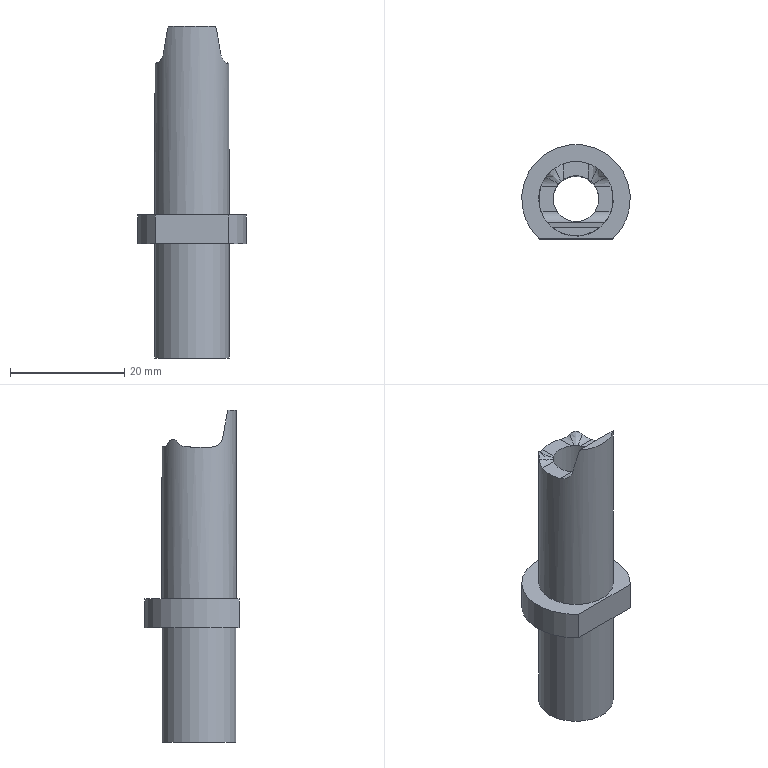Part | STEP file | P011002M015-000 | 1 solid | 20 faces | box 19 x 16.5 x 58.027 mm | volume 4994 mm3 | plane 8 | cylinder 7 | spline 4 | other 1 | commonest cylinder face diameters 4 x3 13 x2 8 x1 19 x1